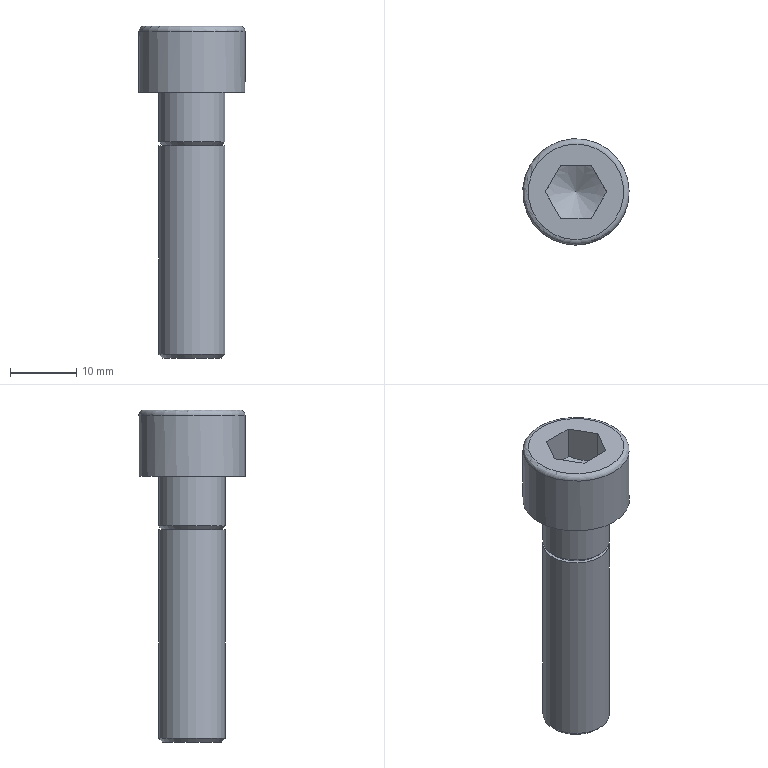Part | STEP file | 1_25 | 1 solid | 17 faces | box 16 x 16 x 50 mm | volume 4802 mm3 | plane 10 | cylinder 3 | cone 3 | torus 1 | commonest cylinder face diameters 10 x2 16 x1